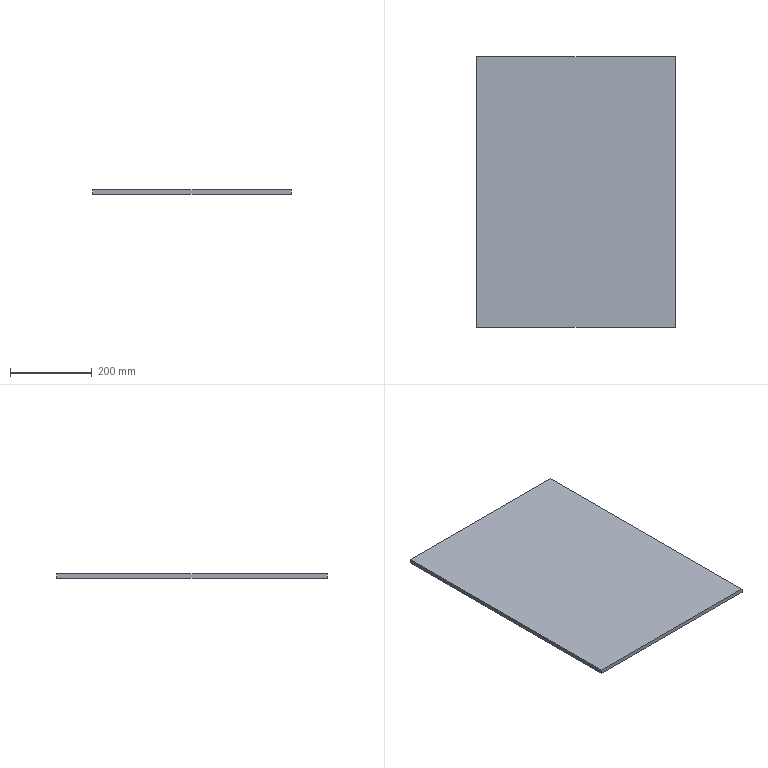Part | STEP file | base da maquina | 1 solid | 6 faces | box 486.837 x 663.677 x 10 mm | volume 3231029 mm3 | plane 6
STEP:
#1=CARTESIAN_POINT('',(0.,0.,0.));
#2=DIRECTION('',(0.,0.,1.));
#3=DIRECTION('',(1.,0.,0.));
#4=AXIS2_PLACEMENT_3D('',#1,#2,#3);
#5=CARTESIAN_POINT('',(-58.066,-180.895,-10.));
#6=VERTEX_POINT('',#5);
#7=CARTESIAN_POINT('',(-58.066,482.783,-10.));
#8=VERTEX_POINT('',#7);
#9=CARTESIAN_POINT('',(-58.066,-180.895,-10.));
#10=DIRECTION('',(0.,1.,0.));
#11=VECTOR('',#10,1.);
#12=LINE('',#9,#11);
#13=CARTESIAN_POINT('',(-58.066,-180.895,0.));
#14=DIRECTION('',(1.,0.,0.));
#15=DIRECTION('',(0.,0.,-1.));
#16=AXIS2_PLACEMENT_3D('',#13,#14,#15);
#17=PLANE('',#16);
#18=CARTESIAN_POINT('',(10.,0.));
#19=DIRECTION('',(0.,1.));
#20=VECTOR('',#19,1.);
#21=LINE('',#18,#20);
#22=(GEOMETRIC_REPRESENTATION_CONTEXT(2)PARAMETRIC_REPRESENTATION_CONTEXT()REPRESENTATION_CONTEXT('',''));
#23=DEFINITIONAL_REPRESENTATION('',(#21),#22);
#24=PCURVE('',#17,#23);
#25=CARTESIAN_POINT('',(-301.485,150.944,-10.));
#26=DIRECTION('',(0.,0.,1.));
#27=DIRECTION('',(1.,0.,0.));
#28=AXIS2_PLACEMENT_3D('',#25,#26,#27);
#29=PLANE('',#28);
#30=CARTESIAN_POINT('',(243.419,-331.839));
#31=DIRECTION('',(0.,1.));
#32=VECTOR('',#31,1.);
#33=LINE('',#30,#32);
#34=(GEOMETRIC_REPRESENTATION_CONTEXT(2)PARAMETRIC_REPRESENTATION_CONTEXT()REPRESENTATION_CONTEXT('',''));
#35=DEFINITIONAL_REPRESENTATION('',(#33),#34);
#36=PCURVE('',#29,#35);
#37=SURFACE_CURVE('',#12,(#24,#36),.PCURVE_S1.);
#38=EDGE_CURVE('',#6,#8,#37,.T.);
#39=ORIENTED_EDGE('',*,*,#38,.T.);
#40=CARTESIAN_POINT('',(-58.066,482.783,0.));
#41=VERTEX_POINT('',#40);
#42=CARTESIAN_POINT('',(-58.066,482.783,0.));
#43=DIRECTION('',(0.,0.,-1.));
#44=VECTOR('',#43,1.);
#45=LINE('',#42,#44);
#46=CARTESIAN_POINT('',(0.,663.677));
#47=DIRECTION('',(1.,0.));
#48=VECTOR('',#47,1.);
#49=LINE('',#46,#48);
#50=(GEOMETRIC_REPRESENTATION_CONTEXT(2)PARAMETRIC_REPRESENTATION_CONTEXT()REPRESENTATION_CONTEXT('',''));
#51=DEFINITIONAL_REPRESENTATION('',(#49),#50);
#52=PCURVE('',#17,#51);
#53=CARTESIAN_POINT('',(-58.066,482.783,0.));
#54=DIRECTION('',(0.,1.,0.));
#55=DIRECTION('',(0.,0.,1.));
#56=AXIS2_PLACEMENT_3D('',#53,#54,#55);
#57=PLANE('',#56);
#58=CARTESIAN_POINT('',(0.,0.));
#59=DIRECTION('',(-1.,0.));
#60=VECTOR('',#59,1.);
#61=LINE('',#58,#60);
#62=(GEOMETRIC_REPRESENTATION_CONTEXT(2)PARAMETRIC_REPRESENTATION_CONTEXT()REPRESENTATION_CONTEXT('',''));
#63=DEFINITIONAL_REPRESENTATION('',(#61),#62);
#64=PCURVE('',#57,#63);
#65=SURFACE_CURVE('',#45,(#52,#64),.PCURVE_S1.);
#66=EDGE_CURVE('',#41,#8,#65,.T.);
#67=ORIENTED_EDGE('',*,*,#66,.F.);
#68=CARTESIAN_POINT('',(-58.066,-180.895,0.));
#69=VERTEX_POINT('',#68);
#70=CARTESIAN_POINT('',(-58.066,482.783,0.));
#71=DIRECTION('',(0.,-1.,0.));
#72=VECTOR('',#71,1.);
#73=LINE('',#70,#72);
#74=CARTESIAN_POINT('',(0.,663.677));
#75=DIRECTION('',(0.,-1.));
#76=VECTOR('',#75,1.);
#77=LINE('',#74,#76);
#78=(GEOMETRIC_REPRESENTATION_CONTEXT(2)PARAMETRIC_REPRESENTATION_CONTEXT()REPRESENTATION_CONTEXT('',''));
#79=DEFINITIONAL_REPRESENTATION('',(#77),#78);
#80=PCURVE('',#17,#79);
#81=CARTESIAN_POINT('',(-301.485,150.944,0.));
#82=DIRECTION('',(0.,0.,1.));
#83=DIRECTION('',(1.,0.,0.));
#84=AXIS2_PLACEMENT_3D('',#81,#82,#83);
#85=PLANE('',#84);
#86=CARTESIAN_POINT('',(243.419,331.839));
#87=DIRECTION('',(0.,-1.));
#88=VECTOR('',#87,1.);
#89=LINE('',#86,#88);
#90=(GEOMETRIC_REPRESENTATION_CONTEXT(2)PARAMETRIC_REPRESENTATION_CONTEXT()REPRESENTATION_CONTEXT('',''));
#91=DEFINITIONAL_REPRESENTATION('',(#89),#90);
#92=PCURVE('',#85,#91);
#93=SURFACE_CURVE('',#73,(#80,#92),.PCURVE_S1.);
#94=EDGE_CURVE('',#41,#69,#93,.T.);
#95=ORIENTED_EDGE('',*,*,#94,.T.);
#96=CARTESIAN_POINT('',(-58.066,-180.895,0.));
#97=DIRECTION('',(0.,0.,-1.));
#98=VECTOR('',#97,1.);
#99=LINE('',#96,#98);
#100=CARTESIAN_POINT('',(0.,0.));
#101=DIRECTION('',(1.,0.));
#102=VECTOR('',#101,1.);
#103=LINE('',#100,#102);
#104=(GEOMETRIC_REPRESENTATION_CONTEXT(2)PARAMETRIC_REPRESENTATION_CONTEXT()REPRESENTATION_CONTEXT('',''));
#105=DEFINITIONAL_REPRESENTATION('',(#103),#104);
#106=PCURVE('',#17,#105);
#107=CARTESIAN_POINT('',(-544.903,-180.895,0.));
#108=DIRECTION('',(0.,-1.,0.));
#109=DIRECTION('',(0.,0.,-1.));
#110=AXIS2_PLACEMENT_3D('',#107,#108,#109);
#111=PLANE('',#110);
#112=CARTESIAN_POINT('',(0.,486.837));
#113=DIRECTION('',(1.,0.));
#114=VECTOR('',#113,1.);
#115=LINE('',#112,#114);
#116=(GEOMETRIC_REPRESENTATION_CONTEXT(2)PARAMETRIC_REPRESENTATION_CONTEXT()REPRESENTATION_CONTEXT('',''));
#117=DEFINITIONAL_REPRESENTATION('',(#115),#116);
#118=PCURVE('',#111,#117);
#119=SURFACE_CURVE('',#99,(#106,#118),.PCURVE_S1.);
#120=EDGE_CURVE('',#69,#6,#119,.T.);
#121=ORIENTED_EDGE('',*,*,#120,.T.);
#122=EDGE_LOOP('',(#39,#67,#95,#121));
#123=FACE_BOUND('',#122,.T.);
#124=ADVANCED_FACE('',(#123),#17,.T.);
#125=CARTESIAN_POINT('',(-544.903,482.783,-10.));
#126=VERTEX_POINT('',#125);
#127=CARTESIAN_POINT('',(-58.066,482.783,-10.));
#128=DIRECTION('',(-1.,0.,0.));
#129=VECTOR('',#128,1.);
#130=LINE('',#127,#129);
#131=CARTESIAN_POINT('',(-10.,0.));
#132=DIRECTION('',(0.,-1.));
#133=VECTOR('',#132,1.);
#134=LINE('',#131,#133);
#135=(GEOMETRIC_REPRESENTATION_CONTEXT(2)PARAMETRIC_REPRESENTATION_CONTEXT()REPRESENTATION_CONTEXT('',''));
#136=DEFINITIONAL_REPRESENTATION('',(#134),#135);
#137=PCURVE('',#57,#136);
#138=CARTESIAN_POINT('',(243.419,331.839));
#139=DIRECTION('',(-1.,0.));
#140=VECTOR('',#139,1.);
#141=LINE('',#138,#140);
#142=(GEOMETRIC_REPRESENTATION_CONTEXT(2)PARAMETRIC_REPRESENTATION_CONTEXT()REPRESENTATION_CONTEXT('',''));
#143=DEFINITIONAL_REPRESENTATION('',(#141),#142);
#144=PCURVE('',#29,#143);
#145=SURFACE_CURVE('',#130,(#137,#144),.PCURVE_S1.);
#146=EDGE_CURVE('',#8,#126,#145,.T.);
#147=ORIENTED_EDGE('',*,*,#146,.T.);
#148=CARTESIAN_POINT('',(-544.903,482.783,0.));
#149=VERTEX_POINT('',#148);
#150=CARTESIAN_POINT('',(-544.903,482.783,0.));
#151=DIRECTION('',(0.,0.,-1.));
#152=VECTOR('',#151,1.);
#153=LINE('',#150,#152);
#154=CARTESIAN_POINT('',(0.,-486.837));
#155=DIRECTION('',(-1.,0.));
#156=VECTOR('',#155,1.);
#157=LINE('',#154,#156);
#158=(GEOMETRIC_REPRESENTATION_CONTEXT(2)PARAMETRIC_REPRESENTATION_CONTEXT()REPRESENTATION_CONTEXT('',''));
#159=DEFINITIONAL_REPRESENTATION('',(#157),#158);
#160=PCURVE('',#57,#159);
#161=CARTESIAN_POINT('',(-544.903,482.783,0.));
#162=DIRECTION('',(-1.,0.,0.));
#163=DIRECTION('',(0.,0.,1.));
#164=AXIS2_PLACEMENT_3D('',#161,#162,#163);
#165=PLANE('',#164);
#166=CARTESIAN_POINT('',(0.,0.));
#167=DIRECTION('',(-1.,0.));
#168=VECTOR('',#167,1.);
#169=LINE('',#166,#168);
#170=(GEOMETRIC_REPRESENTATION_CONTEXT(2)PARAMETRIC_REPRESENTATION_CONTEXT()REPRESENTATION_CONTEXT('',''));
#171=DEFINITIONAL_REPRESENTATION('',(#169),#170);
#172=PCURVE('',#165,#171);
#173=SURFACE_CURVE('',#153,(#160,#172),.PCURVE_S1.);
#174=EDGE_CURVE('',#149,#126,#173,.T.);
#175=ORIENTED_EDGE('',*,*,#174,.F.);
#176=CARTESIAN_POINT('',(-544.903,482.783,0.));
#177=DIRECTION('',(1.,0.,0.));
#178=VECTOR('',#177,1.);
#179=LINE('',#176,#178);
#180=CARTESIAN_POINT('',(0.,-486.837));
#181=DIRECTION('',(0.,1.));
#182=VECTOR('',#181,1.);
#183=LINE('',#180,#182);
#184=(GEOMETRIC_REPRESENTATION_CONTEXT(2)PARAMETRIC_REPRESENTATION_CONTEXT()REPRESENTATION_CONTEXT('',''));
#185=DEFINITIONAL_REPRESENTATION('',(#183),#184);
#186=PCURVE('',#57,#185);
#187=CARTESIAN_POINT('',(-243.419,331.839));
#188=DIRECTION('',(1.,0.));
#189=VECTOR('',#188,1.);
#190=LINE('',#187,#189);
#191=(GEOMETRIC_REPRESENTATION_CONTEXT(2)PARAMETRIC_REPRESENTATION_CONTEXT()REPRESENTATION_CONTEXT('',''));
#192=DEFINITIONAL_REPRESENTATION('',(#190),#191);
#193=PCURVE('',#85,#192);
#194=SURFACE_CURVE('',#179,(#186,#193),.PCURVE_S1.);
#195=EDGE_CURVE('',#149,#41,#194,.T.);
#196=ORIENTED_EDGE('',*,*,#195,.T.);
#197=ORIENTED_EDGE('',*,*,#66,.T.);
#198=EDGE_LOOP('',(#147,#175,#196,#197));
#199=FACE_BOUND('',#198,.T.);
#200=ADVANCED_FACE('',(#199),#57,.T.);
#201=CARTESIAN_POINT('',(-544.903,-180.895,-10.));
#202=VERTEX_POINT('',#201);
#203=CARTESIAN_POINT('',(-544.903,482.783,-10.));
#204=DIRECTION('',(0.,-1.,0.));
#205=VECTOR('',#204,1.);
#206=LINE('',#203,#205);
#207=CARTESIAN_POINT('',(-10.,0.));
#208=DIRECTION('',(0.,-1.));
#209=VECTOR('',#208,1.);
#210=LINE('',#207,#209);
#211=(GEOMETRIC_REPRESENTATION_CONTEXT(2)PARAMETRIC_REPRESENTATION_CONTEXT()REPRESENTATION_CONTEXT('',''));
#212=DEFINITIONAL_REPRESENTATION('',(#210),#211);
#213=PCURVE('',#165,#212);
#214=CARTESIAN_POINT('',(-243.419,331.839));
#215=DIRECTION('',(0.,-1.));
#216=VECTOR('',#215,1.);
#217=LINE('',#214,#216);
#218=(GEOMETRIC_REPRESENTATION_CONTEXT(2)PARAMETRIC_REPRESENTATION_CONTEXT()REPRESENTATION_CONTEXT('',''));
#219=DEFINITIONAL_REPRESENTATION('',(#217),#218);
#220=PCURVE('',#29,#219);
#221=SURFACE_CURVE('',#206,(#213,#220),.PCURVE_S1.);
#222=EDGE_CURVE('',#126,#202,#221,.T.);
#223=ORIENTED_EDGE('',*,*,#222,.T.);
#224=CARTESIAN_POINT('',(-544.903,-180.895,0.));
#225=VERTEX_POINT('',#224);
#226=CARTESIAN_POINT('',(-544.903,-180.895,0.));
#227=DIRECTION('',(0.,0.,-1.));
#228=VECTOR('',#227,1.);
#229=LINE('',#226,#228);
#230=CARTESIAN_POINT('',(0.,-663.677));
#231=DIRECTION('',(-1.,0.));
#232=VECTOR('',#231,1.);
#233=LINE('',#230,#232);
#234=(GEOMETRIC_REPRESENTATION_CONTEXT(2)PARAMETRIC_REPRESENTATION_CONTEXT()REPRESENTATION_CONTEXT('',''));
#235=DEFINITIONAL_REPRESENTATION('',(#233),#234);
#236=PCURVE('',#165,#235);
#237=CARTESIAN_POINT('',(0.,0.));
#238=DIRECTION('',(1.,0.));
#239=VECTOR('',#238,1.);
#240=LINE('',#237,#239);
#241=(GEOMETRIC_REPRESENTATION_CONTEXT(2)PARAMETRIC_REPRESENTATION_CONTEXT()REPRESENTATION_CONTEXT('',''));
#242=DEFINITIONAL_REPRESENTATION('',(#240),#241);
#243=PCURVE('',#111,#242);
#244=SURFACE_CURVE('',#229,(#236,#243),.PCURVE_S1.);
#245=EDGE_CURVE('',#225,#202,#244,.T.);
#246=ORIENTED_EDGE('',*,*,#245,.F.);
#247=CARTESIAN_POINT('',(-544.903,-180.895,0.));
#248=DIRECTION('',(0.,1.,0.));
#249=VECTOR('',#248,1.);
#250=LINE('',#247,#249);
#251=CARTESIAN_POINT('',(0.,-663.677));
#252=DIRECTION('',(0.,1.));
#253=VECTOR('',#252,1.);
#254=LINE('',#251,#253);
#255=(GEOMETRIC_REPRESENTATION_CONTEXT(2)PARAMETRIC_REPRESENTATION_CONTEXT()REPRESENTATION_CONTEXT('',''));
#256=DEFINITIONAL_REPRESENTATION('',(#254),#255);
#257=PCURVE('',#165,#256);
#258=CARTESIAN_POINT('',(-243.419,-331.839));
#259=DIRECTION('',(0.,1.));
#260=VECTOR('',#259,1.);
#261=LINE('',#258,#260);
#262=(GEOMETRIC_REPRESENTATION_CONTEXT(2)PARAMETRIC_REPRESENTATION_CONTEXT()REPRESENTATION_CONTEXT('',''));
#263=DEFINITIONAL_REPRESENTATION('',(#261),#262);
#264=PCURVE('',#85,#263);
#265=SURFACE_CURVE('',#250,(#257,#264),.PCURVE_S1.);
#266=EDGE_CURVE('',#225,#149,#265,.T.);
#267=ORIENTED_EDGE('',*,*,#266,.T.);
#268=ORIENTED_EDGE('',*,*,#174,.T.);
#269=EDGE_LOOP('',(#223,#246,#267,#268));
#270=FACE_BOUND('',#269,.T.);
#271=ADVANCED_FACE('',(#270),#165,.T.);
#272=CARTESIAN_POINT('',(-544.903,-180.895,-10.));
#273=DIRECTION('',(1.,0.,0.));
#274=VECTOR('',#273,1.);
#275=LINE('',#272,#274);
#276=CARTESIAN_POINT('',(10.,0.));
#277=DIRECTION('',(0.,1.));
#278=VECTOR('',#277,1.);
#279=LINE('',#276,#278);
#280=(GEOMETRIC_REPRESENTATION_CONTEXT(2)PARAMETRIC_REPRESENTATION_CONTEXT()REPRESENTATION_CONTEXT('',''));
#281=DEFINITIONAL_REPRESENTATION('',(#279),#280);
#282=PCURVE('',#111,#281);
#283=CARTESIAN_POINT('',(-243.419,-331.839));
#284=DIRECTION('',(1.,0.));
#285=VECTOR('',#284,1.);
#286=LINE('',#283,#285);
#287=(GEOMETRIC_REPRESENTATION_CONTEXT(2)PARAMETRIC_REPRESENTATION_CONTEXT()REPRESENTATION_CONTEXT('',''));
#288=DEFINITIONAL_REPRESENTATION('',(#286),#287);
#289=PCURVE('',#29,#288);
#290=SURFACE_CURVE('',#275,(#282,#289),.PCURVE_S1.);
#291=EDGE_CURVE('',#202,#6,#290,.T.);
#292=ORIENTED_EDGE('',*,*,#291,.T.);
#293=ORIENTED_EDGE('',*,*,#120,.F.);
#294=CARTESIAN_POINT('',(-58.066,-180.895,0.));
#295=DIRECTION('',(-1.,0.,0.));
#296=VECTOR('',#295,1.);
#297=LINE('',#294,#296);
#298=CARTESIAN_POINT('',(0.,486.837));
#299=DIRECTION('',(0.,-1.));
#300=VECTOR('',#299,1.);
#301=LINE('',#298,#300);
#302=(GEOMETRIC_REPRESENTATION_CONTEXT(2)PARAMETRIC_REPRESENTATION_CONTEXT()REPRESENTATION_CONTEXT('',''));
#303=DEFINITIONAL_REPRESENTATION('',(#301),#302);
#304=PCURVE('',#111,#303);
#305=CARTESIAN_POINT('',(243.419,-331.839));
#306=DIRECTION('',(-1.,0.));
#307=VECTOR('',#306,1.);
#308=LINE('',#305,#307);
#309=(GEOMETRIC_REPRESENTATION_CONTEXT(2)PARAMETRIC_REPRESENTATION_CONTEXT()REPRESENTATION_CONTEXT('',''));
#310=DEFINITIONAL_REPRESENTATION('',(#308),#309);
#311=PCURVE('',#85,#310);
#312=SURFACE_CURVE('',#297,(#304,#311),.PCURVE_S1.);
#313=EDGE_CURVE('',#69,#225,#312,.T.);
#314=ORIENTED_EDGE('',*,*,#313,.T.);
#315=ORIENTED_EDGE('',*,*,#245,.T.);
#316=EDGE_LOOP('',(#292,#293,#314,#315));
#317=FACE_BOUND('',#316,.T.);
#318=ADVANCED_FACE('',(#317),#111,.T.);
#319=ORIENTED_EDGE('',*,*,#313,.F.);
#320=ORIENTED_EDGE('',*,*,#94,.F.);
#321=ORIENTED_EDGE('',*,*,#195,.F.);
#322=ORIENTED_EDGE('',*,*,#266,.F.);
#323=EDGE_LOOP('',(#319,#320,#321,#322));
#324=FACE_BOUND('',#323,.T.);
#325=ADVANCED_FACE('',(#324),#85,.T.);
#326=ORIENTED_EDGE('',*,*,#38,.F.);
#327=ORIENTED_EDGE('',*,*,#291,.F.);
#328=ORIENTED_EDGE('',*,*,#222,.F.);
#329=ORIENTED_EDGE('',*,*,#146,.F.);
#330=EDGE_LOOP('',(#326,#327,#328,#329));
#331=FACE_BOUND('',#330,.T.);
#332=ADVANCED_FACE('',(#331),#29,.F.);
#333=CLOSED_SHELL('',(#124,#200,#271,#318,#325,#332));
#334=MANIFOLD_SOLID_BREP('',#333);
#335=(LENGTH_UNIT()NAMED_UNIT(*)SI_UNIT(.MILLI.,.METRE.));
#336=UNCERTAINTY_MEASURE_WITH_UNIT(LENGTH_MEASURE(0.0000001),#335,'','');
#337=(NAMED_UNIT(*)PLANE_ANGLE_UNIT()SI_UNIT($,.RADIAN.));
#338=(NAMED_UNIT(*)SI_UNIT($,.STERADIAN.)SOLID_ANGLE_UNIT());
#339=(GEOMETRIC_REPRESENTATION_CONTEXT(3)GLOBAL_UNCERTAINTY_ASSIGNED_CONTEXT((#336))GLOBAL_UNIT_ASSIGNED_CONTEXT((#335,#337,#338))REPRESENTATION_CONTEXT('',''));
#340=ADVANCED_BREP_SHAPE_REPRESENTATION('',(#4,#334),#339);